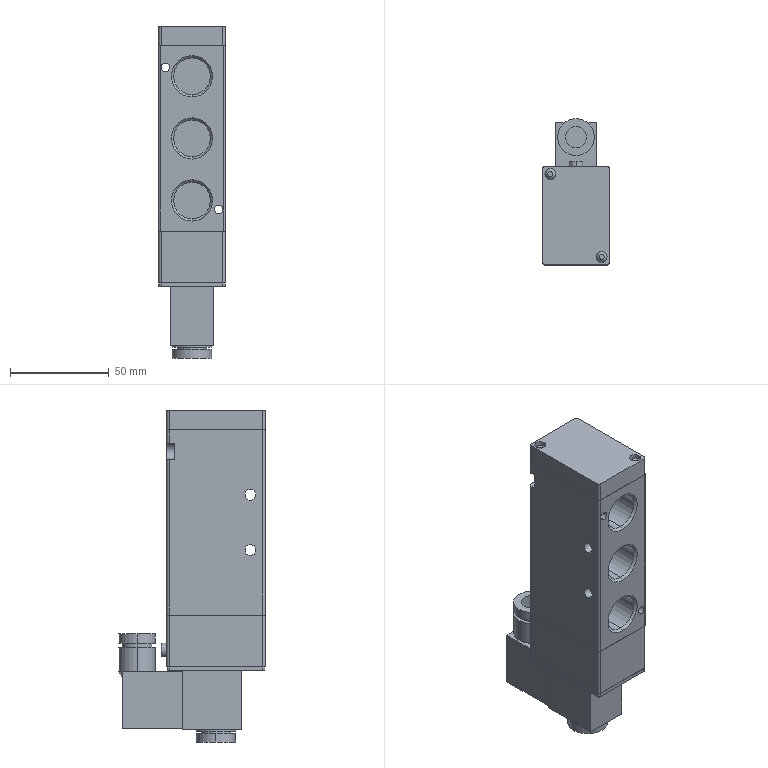Part | SolidWorks | features BaseBody 1 | 1 solid | 123 faces | box 34 x 74.3 x 168.4 mm | volume 241500 mm3 | cylinder 58 | plane 52 | cone 11 | sphere 2 | commonest cylinder face diameters 2.4 x18 18.631 x10 4.3 x4 5.5 x4 5.6 x4 15 x4